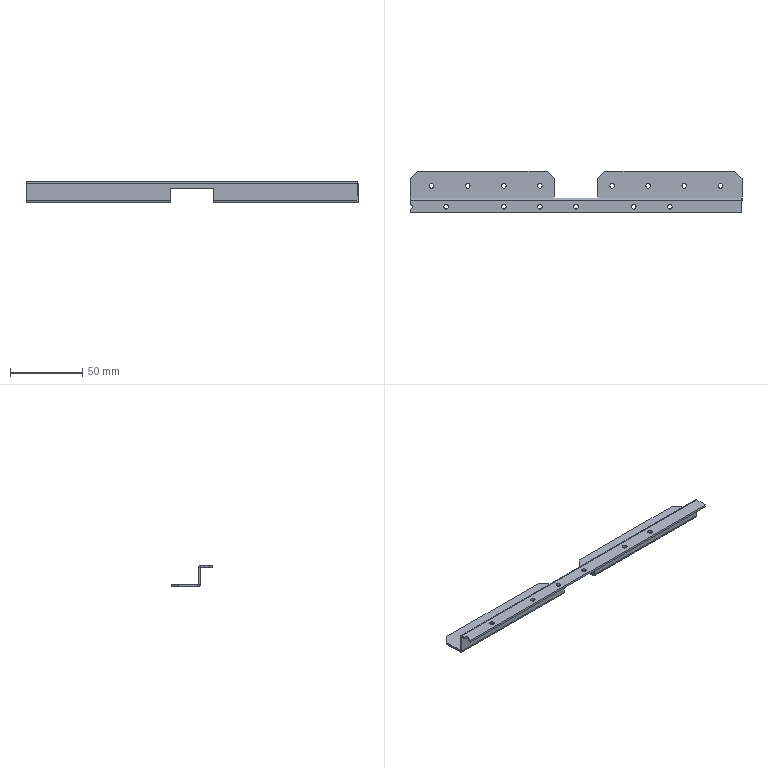Part | SolidWorks | features LPattern 4, ICE 3, EdgeFlange 2, Chamfer 1, FlatPattern 1, SMBaseFlange 1, SheetMetal 1 | 1 solid | 64 faces | box 230 x 28.5 x 15 mm | volume 12722 mm3 | cylinder 35 | plane 29 | commonest cylinder face diameters 3.2 x32 0.2 x3